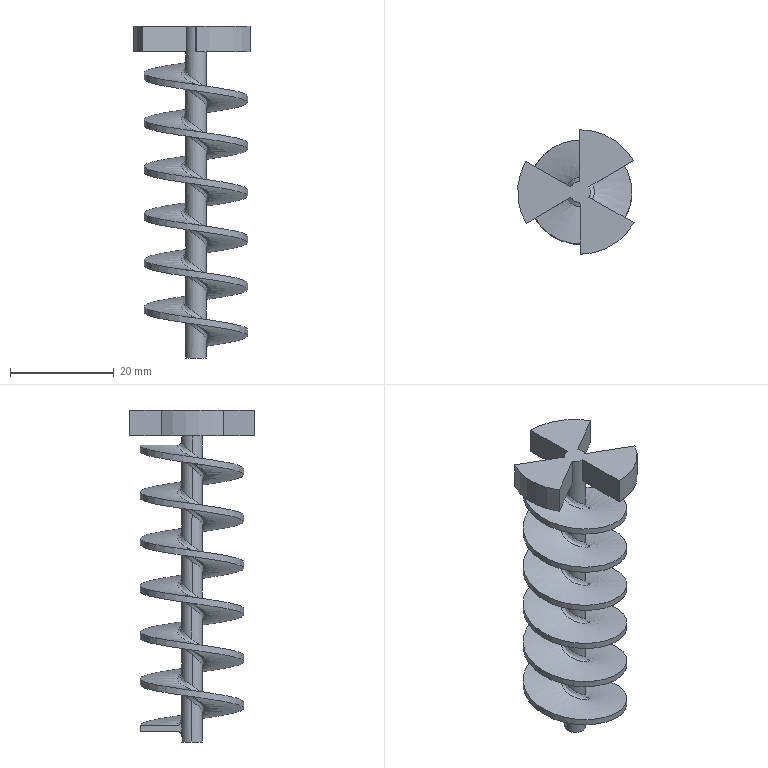Part | SolidWorks | features ICE 2, Extrusion 1, Fillet 1, Helix 1, Sweep 1 | 1 solid | 34 faces | box 22.43 x 24 x 64 mm | volume 4107 mm3 | cylinder 16 | plane 13 | spline 5 | commonest cylinder face diameters 4 x13 24 x3